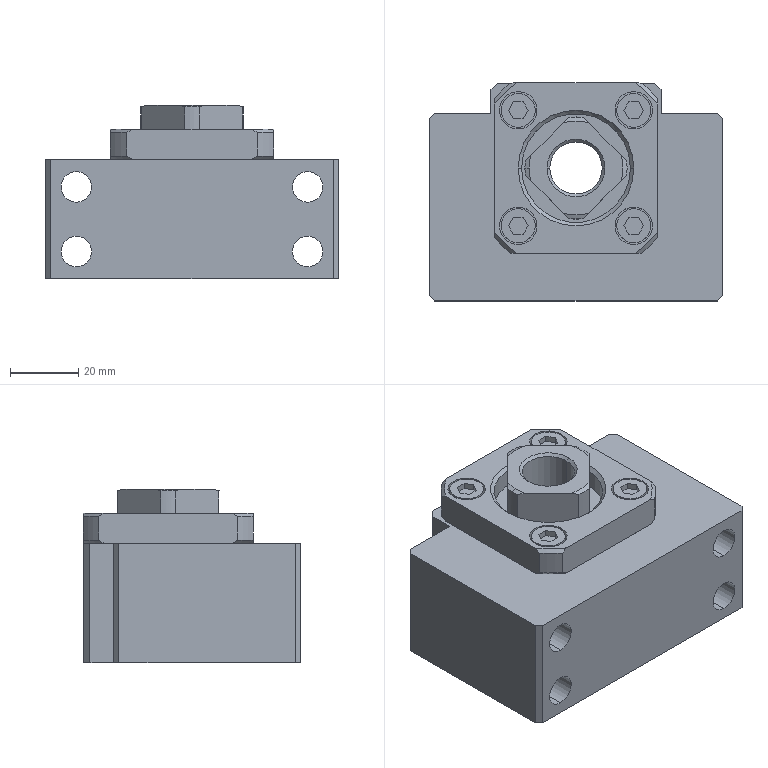Part | SolidWorks | features BaseBody 2 | 2 solids | 184 faces | box 86 x 64 x 51 mm | volume 175508 mm3 | plane 93 | cylinder 63 | spline 28 | commonest cylinder face diameters 9 x8 10 x8 11 x8 14 x8 30 x5 17 x4